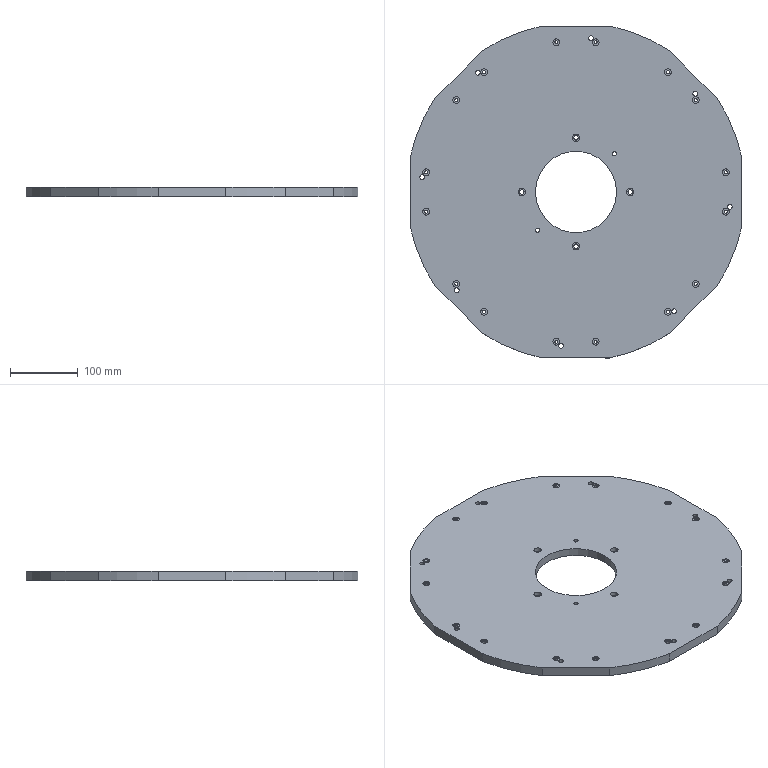Part | STEP file | 11-FG-Z00211 | 1 solid | 271 faces | box 490 x 490 x 14 mm | volume 1970277 mm3 | cylinder 174 | plane 67 | cone 30 | commonest cylinder face diameters 4.5 x32 8 x32 10 x32 20 x20 7 x16 6.6 x8